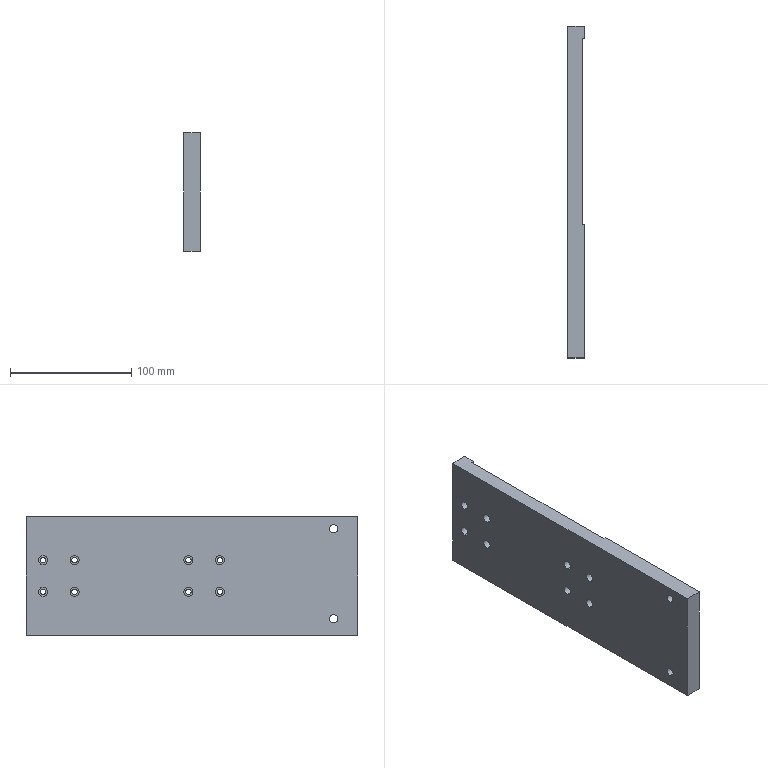Part | Creo | features CURVE 5, CUT 3, DATUM PLANE 3, PROTRUSION 2, COORDINATE SYSTEM 1 | 1 solid | 54 faces | box 14 x 273.995 x 98 mm | volume 341996 mm3 | cylinder 36 | plane 18 | commonest cylinder face diameters 4.5 x16 7.5 x16 6.8 x4